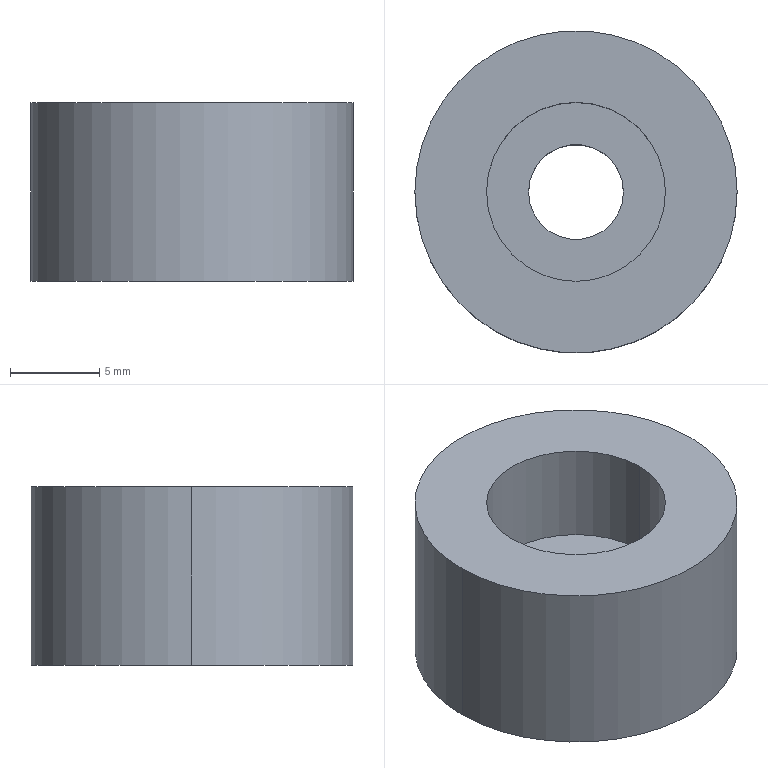Part | STEP file | Buffer block | 1 solid | 9 faces | box 18 x 18 x 10 mm | volume 2002 mm3 | cylinder 6 | plane 3 | commonest cylinder face diameters 5.3 x2 10 x2 18 x2
STEP:
#1=CARTESIAN_POINT('',(0.,0.,0.));
#2=DIRECTION('',(0.,0.,1.));
#3=DIRECTION('',(1.,0.,0.));
#4=AXIS2_PLACEMENT_3D('',#1,#2,#3);
#5=CARTESIAN_POINT('',(5.,0.,4.3));
#6=VERTEX_POINT('',#5);
#7=CARTESIAN_POINT('',(5.,0.,10.));
#8=VERTEX_POINT('',#7);
#9=CARTESIAN_POINT('',(5.,0.,10.));
#10=DIRECTION('',(0.,0.,1.));
#11=VECTOR('',#10,1.);
#12=LINE('',#9,#11);
#13=CARTESIAN_POINT('',(0.,0.,10.));
#14=DIRECTION('',(0.,0.,1.));
#15=DIRECTION('',(1.,0.,0.));
#16=AXIS2_PLACEMENT_3D('',#13,#14,#15);
#17=CYLINDRICAL_SURFACE('',#16,5.);
#18=CARTESIAN_POINT('',(6.283,0.));
#19=DIRECTION('',(0.,1.));
#20=VECTOR('',#19,1.);
#21=LINE('',#18,#20);
#22=(GEOMETRIC_REPRESENTATION_CONTEXT(2)PARAMETRIC_REPRESENTATION_CONTEXT()REPRESENTATION_CONTEXT('',''));
#23=DEFINITIONAL_REPRESENTATION('',(#21),#22);
#24=PCURVE('',#17,#23);
#25=CARTESIAN_POINT('',(0.,0.,10.));
#26=DIRECTION('',(0.,0.,1.));
#27=DIRECTION('',(1.,0.,0.));
#28=AXIS2_PLACEMENT_3D('',#25,#26,#27);
#29=CYLINDRICAL_SURFACE('',#28,5.);
#30=CARTESIAN_POINT('',(0.,0.));
#31=DIRECTION('',(0.,1.));
#32=VECTOR('',#31,1.);
#33=LINE('',#30,#32);
#34=(GEOMETRIC_REPRESENTATION_CONTEXT(2)PARAMETRIC_REPRESENTATION_CONTEXT()REPRESENTATION_CONTEXT('',''));
#35=DEFINITIONAL_REPRESENTATION('',(#33),#34);
#36=PCURVE('',#29,#35);
#37=SURFACE_CURVE('',#12,(#24,#36),.PCURVE_S1.);
#38=EDGE_CURVE('',#6,#8,#37,.T.);
#39=ORIENTED_EDGE('',*,*,#38,.T.);
#40=CARTESIAN_POINT('',(-5.,0.,10.));
#41=VERTEX_POINT('',#40);
#42=CARTESIAN_POINT('',(0.,0.,10.));
#43=DIRECTION('',(0.,0.,1.));
#44=DIRECTION('',(1.,0.,0.));
#45=AXIS2_PLACEMENT_3D('',#42,#43,#44);
#46=CIRCLE('',#45,5.);
#47=CARTESIAN_POINT('',(0.,0.));
#48=DIRECTION('',(1.,0.));
#49=VECTOR('',#48,1.);
#50=LINE('',#47,#49);
#51=(GEOMETRIC_REPRESENTATION_CONTEXT(2)PARAMETRIC_REPRESENTATION_CONTEXT()REPRESENTATION_CONTEXT('',''));
#52=DEFINITIONAL_REPRESENTATION('',(#50),#51);
#53=PCURVE('',#17,#52);
#54=CARTESIAN_POINT('',(0.,0.,10.));
#55=DIRECTION('',(0.,0.,1.));
#56=DIRECTION('',(1.,0.,0.));
#57=AXIS2_PLACEMENT_3D('',#54,#55,#56);
#58=PLANE('',#57);
#59=CARTESIAN_POINT('',(0.,0.));
#60=DIRECTION('',(1.,0.));
#61=AXIS2_PLACEMENT_2D('',#59,#60);
#62=CIRCLE('',#61,5.);
#63=(GEOMETRIC_REPRESENTATION_CONTEXT(2)PARAMETRIC_REPRESENTATION_CONTEXT()REPRESENTATION_CONTEXT('',''));
#64=DEFINITIONAL_REPRESENTATION('',(#62),#63);
#65=PCURVE('',#58,#64);
#66=SURFACE_CURVE('',#46,(#53,#65),.PCURVE_S1.);
#67=EDGE_CURVE('',#41,#8,#66,.T.);
#68=ORIENTED_EDGE('',*,*,#67,.F.);
#69=CARTESIAN_POINT('',(-5.,0.,4.3));
#70=VERTEX_POINT('',#69);
#71=CARTESIAN_POINT('',(-5.,0.,10.));
#72=DIRECTION('',(0.,0.,1.));
#73=VECTOR('',#72,1.);
#74=LINE('',#71,#73);
#75=CARTESIAN_POINT('',(3.142,0.));
#76=DIRECTION('',(0.,1.));
#77=VECTOR('',#76,1.);
#78=LINE('',#75,#77);
#79=(GEOMETRIC_REPRESENTATION_CONTEXT(2)PARAMETRIC_REPRESENTATION_CONTEXT()REPRESENTATION_CONTEXT('',''));
#80=DEFINITIONAL_REPRESENTATION('',(#78),#79);
#81=PCURVE('',#17,#80);
#82=CARTESIAN_POINT('',(3.142,0.));
#83=DIRECTION('',(0.,1.));
#84=VECTOR('',#83,1.);
#85=LINE('',#82,#84);
#86=(GEOMETRIC_REPRESENTATION_CONTEXT(2)PARAMETRIC_REPRESENTATION_CONTEXT()REPRESENTATION_CONTEXT('',''));
#87=DEFINITIONAL_REPRESENTATION('',(#85),#86);
#88=PCURVE('',#29,#87);
#89=SURFACE_CURVE('',#74,(#81,#88),.PCURVE_S1.);
#90=EDGE_CURVE('',#70,#41,#89,.T.);
#91=ORIENTED_EDGE('',*,*,#90,.F.);
#92=CARTESIAN_POINT('',(0.,0.,4.3));
#93=DIRECTION('',(0.,0.,1.));
#94=DIRECTION('',(1.,0.,0.));
#95=AXIS2_PLACEMENT_3D('',#92,#93,#94);
#96=CIRCLE('',#95,5.);
#97=CARTESIAN_POINT('',(0.,-5.7));
#98=DIRECTION('',(1.,0.));
#99=VECTOR('',#98,1.);
#100=LINE('',#97,#99);
#101=(GEOMETRIC_REPRESENTATION_CONTEXT(2)PARAMETRIC_REPRESENTATION_CONTEXT()REPRESENTATION_CONTEXT('',''));
#102=DEFINITIONAL_REPRESENTATION('',(#100),#101);
#103=PCURVE('',#17,#102);
#104=CARTESIAN_POINT('',(2.65,0.,4.3));
#105=DIRECTION('',(0.,0.,-1.));
#106=DIRECTION('',(-1.,0.,0.));
#107=AXIS2_PLACEMENT_3D('',#104,#105,#106);
#108=PLANE('',#107);
#109=CARTESIAN_POINT('',(-2.35,0.));
#110=CARTESIAN_POINT('',(-2.35,8.66));
#111=CARTESIAN_POINT('',(5.15,4.33));
#112=CARTESIAN_POINT('',(12.65,0.));
#113=CARTESIAN_POINT('',(5.15,-4.33));
#114=CARTESIAN_POINT('',(-2.35,-8.66));
#115=CARTESIAN_POINT('',(-2.35,0.));
#116=(BOUNDED_CURVE()B_SPLINE_CURVE(2,(#109,#110,#111,#112,#113,#114,#115),.UNSPECIFIED.,.T.,.F.)B_SPLINE_CURVE_WITH_KNOTS((1,2,2,2,2,1),(-2.094,0.,2.094,4.189,6.283,8.378),.UNSPECIFIED.)CURVE()GEOMETRIC_REPRESENTATION_ITEM()RATIONAL_B_SPLINE_CURVE((1.,0.5,1.,0.5,1.,0.5,1.))REPRESENTATION_ITEM(''));
#117=(GEOMETRIC_REPRESENTATION_CONTEXT(2)PARAMETRIC_REPRESENTATION_CONTEXT()REPRESENTATION_CONTEXT('',''));
#118=DEFINITIONAL_REPRESENTATION('',(#116),#117);
#119=PCURVE('',#108,#118);
#120=SURFACE_CURVE('',#96,(#103,#119),.PCURVE_S1.);
#121=EDGE_CURVE('',#70,#6,#120,.T.);
#122=ORIENTED_EDGE('',*,*,#121,.T.);
#123=EDGE_LOOP('',(#39,#68,#91,#122));
#124=FACE_BOUND('',#123,.F.);
#125=ADVANCED_FACE('',(#124),#17,.F.);
#126=CARTESIAN_POINT('',(2.65,0.,0.));
#127=VERTEX_POINT('',#126);
#128=CARTESIAN_POINT('',(2.65,0.,4.3));
#129=VERTEX_POINT('',#128);
#130=CARTESIAN_POINT('',(2.65,0.,10.));
#131=DIRECTION('',(0.,0.,1.));
#132=VECTOR('',#131,1.);
#133=LINE('',#130,#132);
#134=CARTESIAN_POINT('',(0.,0.,10.));
#135=DIRECTION('',(0.,0.,1.));
#136=DIRECTION('',(1.,0.,0.));
#137=AXIS2_PLACEMENT_3D('',#134,#135,#136);
#138=CYLINDRICAL_SURFACE('',#137,2.65);
#139=CARTESIAN_POINT('',(6.283,0.));
#140=DIRECTION('',(0.,1.));
#141=VECTOR('',#140,1.);
#142=LINE('',#139,#141);
#143=(GEOMETRIC_REPRESENTATION_CONTEXT(2)PARAMETRIC_REPRESENTATION_CONTEXT()REPRESENTATION_CONTEXT('',''));
#144=DEFINITIONAL_REPRESENTATION('',(#142),#143);
#145=PCURVE('',#138,#144);
#146=CARTESIAN_POINT('',(0.,0.,10.));
#147=DIRECTION('',(0.,0.,1.));
#148=DIRECTION('',(1.,0.,0.));
#149=AXIS2_PLACEMENT_3D('',#146,#147,#148);
#150=CYLINDRICAL_SURFACE('',#149,2.65);
#151=CARTESIAN_POINT('',(0.,0.));
#152=DIRECTION('',(0.,1.));
#153=VECTOR('',#152,1.);
#154=LINE('',#151,#153);
#155=(GEOMETRIC_REPRESENTATION_CONTEXT(2)PARAMETRIC_REPRESENTATION_CONTEXT()REPRESENTATION_CONTEXT('',''));
#156=DEFINITIONAL_REPRESENTATION('',(#154),#155);
#157=PCURVE('',#150,#156);
#158=SURFACE_CURVE('',#133,(#145,#157),.PCURVE_S1.);
#159=EDGE_CURVE('',#127,#129,#158,.T.);
#160=ORIENTED_EDGE('',*,*,#159,.T.);
#161=CARTESIAN_POINT('',(-2.65,0.,4.3));
#162=VERTEX_POINT('',#161);
#163=CARTESIAN_POINT('',(0.,0.,4.3));
#164=DIRECTION('',(0.,0.,1.));
#165=DIRECTION('',(1.,0.,0.));
#166=AXIS2_PLACEMENT_3D('',#163,#164,#165);
#167=CIRCLE('',#166,2.65);
#168=CARTESIAN_POINT('',(0.,-5.7));
#169=DIRECTION('',(1.,0.));
#170=VECTOR('',#169,1.);
#171=LINE('',#168,#170);
#172=(GEOMETRIC_REPRESENTATION_CONTEXT(2)PARAMETRIC_REPRESENTATION_CONTEXT()REPRESENTATION_CONTEXT('',''));
#173=DEFINITIONAL_REPRESENTATION('',(#171),#172);
#174=PCURVE('',#138,#173);
#175=CARTESIAN_POINT('',(0.,0.));
#176=CARTESIAN_POINT('',(0.,4.59));
#177=CARTESIAN_POINT('',(3.975,2.295));
#178=CARTESIAN_POINT('',(7.95,0.));
#179=CARTESIAN_POINT('',(3.975,-2.295));
#180=CARTESIAN_POINT('',(0.,-4.59));
#181=CARTESIAN_POINT('',(0.,0.));
#182=(BOUNDED_CURVE()B_SPLINE_CURVE(2,(#175,#176,#177,#178,#179,#180,#181),.UNSPECIFIED.,.T.,.F.)B_SPLINE_CURVE_WITH_KNOTS((1,2,2,2,2,1),(-2.094,0.,2.094,4.189,6.283,8.378),.UNSPECIFIED.)CURVE()GEOMETRIC_REPRESENTATION_ITEM()RATIONAL_B_SPLINE_CURVE((1.,0.5,1.,0.5,1.,0.5,1.))REPRESENTATION_ITEM(''));
#183=(GEOMETRIC_REPRESENTATION_CONTEXT(2)PARAMETRIC_REPRESENTATION_CONTEXT()REPRESENTATION_CONTEXT('',''));
#184=DEFINITIONAL_REPRESENTATION('',(#182),#183);
#185=PCURVE('',#108,#184);
#186=SURFACE_CURVE('',#167,(#174,#185),.PCURVE_S1.);
#187=EDGE_CURVE('',#162,#129,#186,.T.);
#188=ORIENTED_EDGE('',*,*,#187,.F.);
#189=CARTESIAN_POINT('',(-2.65,0.,0.));
#190=VERTEX_POINT('',#189);
#191=CARTESIAN_POINT('',(-2.65,0.,10.));
#192=DIRECTION('',(0.,0.,1.));
#193=VECTOR('',#192,1.);
#194=LINE('',#191,#193);
#195=CARTESIAN_POINT('',(3.142,0.));
#196=DIRECTION('',(0.,1.));
#197=VECTOR('',#196,1.);
#198=LINE('',#195,#197);
#199=(GEOMETRIC_REPRESENTATION_CONTEXT(2)PARAMETRIC_REPRESENTATION_CONTEXT()REPRESENTATION_CONTEXT('',''));
#200=DEFINITIONAL_REPRESENTATION('',(#198),#199);
#201=PCURVE('',#138,#200);
#202=CARTESIAN_POINT('',(3.142,0.));
#203=DIRECTION('',(0.,1.));
#204=VECTOR('',#203,1.);
#205=LINE('',#202,#204);
#206=(GEOMETRIC_REPRESENTATION_CONTEXT(2)PARAMETRIC_REPRESENTATION_CONTEXT()REPRESENTATION_CONTEXT('',''));
#207=DEFINITIONAL_REPRESENTATION('',(#205),#206);
#208=PCURVE('',#150,#207);
#209=SURFACE_CURVE('',#194,(#201,#208),.PCURVE_S1.);
#210=EDGE_CURVE('',#190,#162,#209,.T.);
#211=ORIENTED_EDGE('',*,*,#210,.F.);
#212=CARTESIAN_POINT('',(0.,0.,0.));
#213=DIRECTION('',(0.,0.,1.));
#214=DIRECTION('',(1.,0.,0.));
#215=AXIS2_PLACEMENT_3D('',#212,#213,#214);
#216=CIRCLE('',#215,2.65);
#217=CARTESIAN_POINT('',(0.,-10.));
#218=DIRECTION('',(1.,0.));
#219=VECTOR('',#218,1.);
#220=LINE('',#217,#219);
#221=(GEOMETRIC_REPRESENTATION_CONTEXT(2)PARAMETRIC_REPRESENTATION_CONTEXT()REPRESENTATION_CONTEXT('',''));
#222=DEFINITIONAL_REPRESENTATION('',(#220),#221);
#223=PCURVE('',#138,#222);
#224=CARTESIAN_POINT('',(0.,0.,0.));
#225=DIRECTION('',(0.,0.,1.));
#226=DIRECTION('',(1.,0.,0.));
#227=AXIS2_PLACEMENT_3D('',#224,#225,#226);
#228=PLANE('',#227);
#229=CARTESIAN_POINT('',(0.,0.));
#230=DIRECTION('',(1.,0.));
#231=AXIS2_PLACEMENT_2D('',#229,#230);
#232=CIRCLE('',#231,2.65);
#233=(GEOMETRIC_REPRESENTATION_CONTEXT(2)PARAMETRIC_REPRESENTATION_CONTEXT()REPRESENTATION_CONTEXT('',''));
#234=DEFINITIONAL_REPRESENTATION('',(#232),#233);
#235=PCURVE('',#228,#234);
#236=SURFACE_CURVE('',#216,(#223,#235),.PCURVE_S1.);
#237=EDGE_CURVE('',#190,#127,#236,.T.);
#238=ORIENTED_EDGE('',*,*,#237,.T.);
#239=EDGE_LOOP('',(#160,#188,#211,#238));
#240=FACE_BOUND('',#239,.F.);
#241=ADVANCED_FACE('',(#240),#138,.F.);
#242=CARTESIAN_POINT('',(9.,0.,10.));
#243=VERTEX_POINT('',#242);
#244=CARTESIAN_POINT('',(-9.,0.,10.));
#245=VERTEX_POINT('',#244);
#246=CARTESIAN_POINT('',(0.,0.,10.));
#247=DIRECTION('',(0.,0.,1.));
#248=DIRECTION('',(1.,0.,0.));
#249=AXIS2_PLACEMENT_3D('',#246,#247,#248);
#250=CIRCLE('',#249,9.);
#251=CARTESIAN_POINT('',(0.,0.,10.));
#252=DIRECTION('',(0.,0.,-1.));
#253=DIRECTION('',(-1.,0.,0.));
#254=AXIS2_PLACEMENT_3D('',#251,#252,#253);
#255=CYLINDRICAL_SURFACE('',#254,9.);
#256=CARTESIAN_POINT('',(3.142,0.));
#257=DIRECTION('',(-1.,0.));
#258=VECTOR('',#257,1.);
#259=LINE('',#256,#258);
#260=(GEOMETRIC_REPRESENTATION_CONTEXT(2)PARAMETRIC_REPRESENTATION_CONTEXT()REPRESENTATION_CONTEXT('',''));
#261=DEFINITIONAL_REPRESENTATION('',(#259),#260);
#262=PCURVE('',#255,#261);
#263=CARTESIAN_POINT('',(0.,0.));
#264=DIRECTION('',(1.,0.));
#265=AXIS2_PLACEMENT_2D('',#263,#264);
#266=CIRCLE('',#265,9.);
#267=(GEOMETRIC_REPRESENTATION_CONTEXT(2)PARAMETRIC_REPRESENTATION_CONTEXT()REPRESENTATION_CONTEXT('',''));
#268=DEFINITIONAL_REPRESENTATION('',(#266),#267);
#269=PCURVE('',#58,#268);
#270=SURFACE_CURVE('',#250,(#262,#269),.PCURVE_S1.);
#271=EDGE_CURVE('',#243,#245,#270,.T.);
#272=ORIENTED_EDGE('',*,*,#271,.F.);
#273=CARTESIAN_POINT('',(9.,0.,0.));
#274=VERTEX_POINT('',#273);
#275=CARTESIAN_POINT('',(9.,0.,10.));
#276=DIRECTION('',(0.,0.,-1.));
#277=VECTOR('',#276,1.);
#278=LINE('',#275,#277);
#279=CARTESIAN_POINT('',(3.142,0.));
#280=DIRECTION('',(0.,1.));
#281=VECTOR('',#280,1.);
#282=LINE('',#279,#281);
#283=(GEOMETRIC_REPRESENTATION_CONTEXT(2)PARAMETRIC_REPRESENTATION_CONTEXT()REPRESENTATION_CONTEXT('',''));
#284=DEFINITIONAL_REPRESENTATION('',(#282),#283);
#285=PCURVE('',#255,#284);
#286=CARTESIAN_POINT('',(0.,0.,10.));
#287=DIRECTION('',(0.,0.,-1.));
#288=DIRECTION('',(-1.,0.,0.));
#289=AXIS2_PLACEMENT_3D('',#286,#287,#288);
#290=CYLINDRICAL_SURFACE('',#289,9.);
#291=CARTESIAN_POINT('',(3.142,0.));
#292=DIRECTION('',(0.,1.));
#293=VECTOR('',#292,1.);
#294=LINE('',#291,#293);
#295=(GEOMETRIC_REPRESENTATION_CONTEXT(2)PARAMETRIC_REPRESENTATION_CONTEXT()REPRESENTATION_CONTEXT('',''));
#296=DEFINITIONAL_REPRESENTATION('',(#294),#295);
#297=PCURVE('',#290,#296);
#298=SURFACE_CURVE('',#278,(#285,#297),.PCURVE_S1.);
#299=EDGE_CURVE('',#243,#274,#298,.T.);
#300=ORIENTED_EDGE('',*,*,#299,.T.);
#301=CARTESIAN_POINT('',(-9.,0.,0.));
#302=VERTEX_POINT('',#301);
#303=CARTESIAN_POINT('',(0.,0.,0.));
#304=DIRECTION('',(0.,0.,1.));
#305=DIRECTION('',(1.,0.,0.));
#306=AXIS2_PLACEMENT_3D('',#303,#304,#305);
#307=CIRCLE('',#306,9.);
#308=CARTESIAN_POINT('',(3.142,10.));
#309=DIRECTION('',(-1.,0.));
#310=VECTOR('',#309,1.);
#311=LINE('',#308,#310);
#312=(GEOMETRIC_REPRESENTATION_CONTEXT(2)PARAMETRIC_REPRESENTATION_CONTEXT()REPRESENTATION_CONTEXT('',''));
#313=DEFINITIONAL_REPRESENTATION('',(#311),#312);
#314=PCURVE('',#255,#313);
#315=CARTESIAN_POINT('',(0.,0.));
#316=DIRECTION('',(1.,0.));
#317=AXIS2_PLACEMENT_2D('',#315,#316);
#318=CIRCLE('',#317,9.);
#319=(GEOMETRIC_REPRESENTATION_CONTEXT(2)PARAMETRIC_REPRESENTATION_CONTEXT()REPRESENTATION_CONTEXT('',''));
#320=DEFINITIONAL_REPRESENTATION('',(#318),#319);
#321=PCURVE('',#228,#320);
#322=SURFACE_CURVE('',#307,(#314,#321),.PCURVE_S1.);
#323=EDGE_CURVE('',#274,#302,#322,.T.);
#324=ORIENTED_EDGE('',*,*,#323,.T.);
#325=CARTESIAN_POINT('',(-9.,0.,10.));
#326=DIRECTION('',(0.,0.,-1.));
#327=VECTOR('',#326,1.);
#328=LINE('',#325,#327);
#329=CARTESIAN_POINT('',(0.,0.));
#330=DIRECTION('',(0.,1.));
#331=VECTOR('',#330,1.);
#332=LINE('',#329,#331);
#333=(GEOMETRIC_REPRESENTATION_CONTEXT(2)PARAMETRIC_REPRESENTATION_CONTEXT()REPRESENTATION_CONTEXT('',''));
#334=DEFINITIONAL_REPRESENTATION('',(#332),#333);
#335=PCURVE('',#255,#334);
#336=CARTESIAN_POINT('',(6.283,0.));
#337=DIRECTION('',(0.,1.));
#338=VECTOR('',#337,1.);
#339=LINE('',#336,#338);
#340=(GEOMETRIC_REPRESENTATION_CONTEXT(2)PARAMETRIC_REPRESENTATION_CONTEXT()REPRESENTATION_CONTEXT('',''));
#341=DEFINITIONAL_REPRESENTATION('',(#339),#340);
#342=PCURVE('',#290,#341);
#343=SURFACE_CURVE('',#328,(#335,#342),.PCURVE_S1.);
#344=EDGE_CURVE('',#245,#302,#343,.T.);
#345=ORIENTED_EDGE('',*,*,#344,.F.);
#346=EDGE_LOOP('',(#272,#300,#324,#345));
#347=FACE_BOUND('',#346,.T.);
#348=ADVANCED_FACE('',(#347),#255,.T.);
#349=ORIENTED_EDGE('',*,*,#299,.F.);
#350=CARTESIAN_POINT('',(0.,0.,10.));
#351=DIRECTION('',(0.,0.,1.));
#352=DIRECTION('',(1.,0.,0.));
#353=AXIS2_PLACEMENT_3D('',#350,#351,#352);
#354=CIRCLE('',#353,9.);
#355=CARTESIAN_POINT('',(9.425,0.));
#356=DIRECTION('',(-1.,0.));
#357=VECTOR('',#356,1.);
#358=LINE('',#355,#357);
#359=(GEOMETRIC_REPRESENTATION_CONTEXT(2)PARAMETRIC_REPRESENTATION_CONTEXT()REPRESENTATION_CONTEXT('',''));
#360=DEFINITIONAL_REPRESENTATION('',(#358),#359);
#361=PCURVE('',#290,#360);
#362=CARTESIAN_POINT('',(0.,0.));
#363=DIRECTION('',(1.,0.));
#364=AXIS2_PLACEMENT_2D('',#362,#363);
#365=CIRCLE('',#364,9.);
#366=(GEOMETRIC_REPRESENTATION_CONTEXT(2)PARAMETRIC_REPRESENTATION_CONTEXT()REPRESENTATION_CONTEXT('',''));
#367=DEFINITIONAL_REPRESENTATION('',(#365),#366);
#368=PCURVE('',#58,#367);
#369=SURFACE_CURVE('',#354,(#361,#368),.PCURVE_S1.);
#370=EDGE_CURVE('',#245,#243,#369,.T.);
#371=ORIENTED_EDGE('',*,*,#370,.F.);
#372=ORIENTED_EDGE('',*,*,#344,.T.);
#373=CARTESIAN_POINT('',(0.,0.,0.));
#374=DIRECTION('',(0.,0.,1.));
#375=DIRECTION('',(1.,0.,0.));
#376=AXIS2_PLACEMENT_3D('',#373,#374,#375);
#377=CIRCLE('',#376,9.);
#378=CARTESIAN_POINT('',(9.425,10.));
#379=DIRECTION('',(-1.,0.));
#380=VECTOR('',#379,1.);
#381=LINE('',#378,#380);
#382=(GEOMETRIC_REPRESENTATION_CONTEXT(2)PARAMETRIC_REPRESENTATION_CONTEXT()REPRESENTATION_CONTEXT('',''));
#383=DEFINITIONAL_REPRESENTATION('',(#381),#382);
#384=PCURVE('',#290,#383);
#385=CARTESIAN_POINT('',(0.,0.));
#386=DIRECTION('',(1.,0.));
#387=AXIS2_PLACEMENT_2D('',#385,#386);
#388=CIRCLE('',#387,9.);
#389=(GEOMETRIC_REPRESENTATION_CONTEXT(2)PARAMETRIC_REPRESENTATION_CONTEXT()REPRESENTATION_CONTEXT('',''));
#390=DEFINITIONAL_REPRESENTATION('',(#388),#389);
#391=PCURVE('',#228,#390);
#392=SURFACE_CURVE('',#377,(#384,#391),.PCURVE_S1.);
#393=EDGE_CURVE('',#302,#274,#392,.T.);
#394=ORIENTED_EDGE('',*,*,#393,.T.);
#395=EDGE_LOOP('',(#349,#371,#372,#394));
#396=FACE_BOUND('',#395,.T.);
#397=ADVANCED_FACE('',(#396),#290,.T.);
#398=CARTESIAN_POINT('',(0.,0.,10.));
#399=DIRECTION('',(0.,0.,1.));
#400=DIRECTION('',(1.,0.,0.));
#401=AXIS2_PLACEMENT_3D('',#398,#399,#400);
#402=CIRCLE('',#401,5.);
#403=CARTESIAN_POINT('',(0.,0.));
#404=DIRECTION('',(1.,0.));
#405=AXIS2_PLACEMENT_2D('',#403,#404);
#406=CIRCLE('',#405,5.);
#407=(GEOMETRIC_REPRESENTATION_CONTEXT(2)PARAMETRIC_REPRESENTATION_CONTEXT()REPRESENTATION_CONTEXT('',''));
#408=DEFINITIONAL_REPRESENTATION('',(#406),#407);
#409=PCURVE('',#58,#408);
#410=CARTESIAN_POINT('',(0.,0.));
#411=DIRECTION('',(1.,0.));
#412=VECTOR('',#411,1.);
#413=LINE('',#410,#412);
#414=(GEOMETRIC_REPRESENTATION_CONTEXT(2)PARAMETRIC_REPRESENTATION_CONTEXT()REPRESENTATION_CONTEXT('',''));
#415=DEFINITIONAL_REPRESENTATION('',(#413),#414);
#416=PCURVE('',#29,#415);
#417=SURFACE_CURVE('',#402,(#409,#416),.PCURVE_S1.);
#418=EDGE_CURVE('',#8,#41,#417,.T.);
#419=ORIENTED_EDGE('',*,*,#418,.F.);
#420=ORIENTED_EDGE('',*,*,#67,.F.);
#421=EDGE_LOOP('',(#419,#420));
#422=FACE_BOUND('',#421,.T.);
#423=ORIENTED_EDGE('',*,*,#370,.T.);
#424=ORIENTED_EDGE('',*,*,#271,.T.);
#425=EDGE_LOOP('',(#423,#424));
#426=FACE_BOUND('',#425,.T.);
#427=ADVANCED_FACE('',(#422,#426),#58,.T.);
#428=CARTESIAN_POINT('',(0.,0.,0.));
#429=DIRECTION('',(0.,0.,1.));
#430=DIRECTION('',(1.,0.,0.));
#431=AXIS2_PLACEMENT_3D('',#428,#429,#430);
#432=CIRCLE('',#431,2.65);
#433=CARTESIAN_POINT('',(0.,0.));
#434=DIRECTION('',(1.,0.));
#435=AXIS2_PLACEMENT_2D('',#433,#434);
#436=CIRCLE('',#435,2.65);
#437=(GEOMETRIC_REPRESENTATION_CONTEXT(2)PARAMETRIC_REPRESENTATION_CONTEXT()REPRESENTATION_CONTEXT('',''));
#438=DEFINITIONAL_REPRESENTATION('',(#436),#437);
#439=PCURVE('',#228,#438);
#440=CARTESIAN_POINT('',(0.,-10.));
#441=DIRECTION('',(1.,0.));
#442=VECTOR('',#441,1.);
#443=LINE('',#440,#442);
#444=(GEOMETRIC_REPRESENTATION_CONTEXT(2)PARAMETRIC_REPRESENTATION_CONTEXT()REPRESENTATION_CONTEXT('',''));
#445=DEFINITIONAL_REPRESENTATION('',(#443),#444);
#446=PCURVE('',#150,#445);
#447=SURFACE_CURVE('',#432,(#439,#446),.PCURVE_S1.);
#448=EDGE_CURVE('',#127,#190,#447,.T.);
#449=ORIENTED_EDGE('',*,*,#448,.T.);
#450=ORIENTED_EDGE('',*,*,#237,.T.);
#451=EDGE_LOOP('',(#449,#450));
#452=FACE_BOUND('',#451,.T.);
#453=ORIENTED_EDGE('',*,*,#393,.F.);
#454=ORIENTED_EDGE('',*,*,#323,.F.);
#455=EDGE_LOOP('',(#453,#454));
#456=FACE_BOUND('',#455,.T.);
#457=ADVANCED_FACE('',(#452,#456),#228,.F.);
#458=CARTESIAN_POINT('',(0.,0.,4.3));
#459=DIRECTION('',(0.,0.,1.));
#460=DIRECTION('',(1.,0.,0.));
#461=AXIS2_PLACEMENT_3D('',#458,#459,#460);
#462=CIRCLE('',#461,2.65);
#463=CARTESIAN_POINT('',(0.,-5.7));
#464=DIRECTION('',(1.,0.));
#465=VECTOR('',#464,1.);
#466=LINE('',#463,#465);
#467=(GEOMETRIC_REPRESENTATION_CONTEXT(2)PARAMETRIC_REPRESENTATION_CONTEXT()REPRESENTATION_CONTEXT('',''));
#468=DEFINITIONAL_REPRESENTATION('',(#466),#467);
#469=PCURVE('',#150,#468);
#470=CARTESIAN_POINT('',(0.,0.));
#471=CARTESIAN_POINT('',(0.,4.59));
#472=CARTESIAN_POINT('',(3.975,2.295));
#473=CARTESIAN_POINT('',(7.95,0.));
#474=CARTESIAN_POINT('',(3.975,-2.295));
#475=CARTESIAN_POINT('',(0.,-4.59));
#476=CARTESIAN_POINT('',(0.,0.));
#477=(BOUNDED_CURVE()B_SPLINE_CURVE(2,(#470,#471,#472,#473,#474,#475,#476),.UNSPECIFIED.,.T.,.F.)B_SPLINE_CURVE_WITH_KNOTS((1,2,2,2,2,1),(-2.094,0.,2.094,4.189,6.283,8.378),.UNSPECIFIED.)CURVE()GEOMETRIC_REPRESENTATION_ITEM()RATIONAL_B_SPLINE_CURVE((1.,0.5,1.,0.5,1.,0.5,1.))REPRESENTATION_ITEM(''));
#478=(GEOMETRIC_REPRESENTATION_CONTEXT(2)PARAMETRIC_REPRESENTATION_CONTEXT()REPRESENTATION_CONTEXT('',''));
#479=DEFINITIONAL_REPRESENTATION('',(#477),#478);
#480=PCURVE('',#108,#479);
#481=SURFACE_CURVE('',#462,(#469,#480),.PCURVE_S1.);
#482=EDGE_CURVE('',#129,#162,#481,.T.);
#483=ORIENTED_EDGE('',*,*,#482,.F.);
#484=ORIENTED_EDGE('',*,*,#159,.F.);
#485=ORIENTED_EDGE('',*,*,#448,.T.);
#486=ORIENTED_EDGE('',*,*,#210,.T.);
#487=EDGE_LOOP('',(#483,#484,#485,#486));
#488=FACE_BOUND('',#487,.F.);
#489=ADVANCED_FACE('',(#488),#150,.F.);
#490=ORIENTED_EDGE('',*,*,#482,.F.);
#491=ORIENTED_EDGE('',*,*,#187,.F.);
#492=EDGE_LOOP('',(#490,#491));
#493=FACE_BOUND('',#492,.T.);
#494=CARTESIAN_POINT('',(0.,0.,4.3));
#495=DIRECTION('',(0.,0.,1.));
#496=DIRECTION('',(1.,0.,0.));
#497=AXIS2_PLACEMENT_3D('',#494,#495,#496);
#498=CIRCLE('',#497,5.);
#499=CARTESIAN_POINT('',(-2.35,0.));
#500=CARTESIAN_POINT('',(-2.35,8.66));
#501=CARTESIAN_POINT('',(5.15,4.33));
#502=CARTESIAN_POINT('',(12.65,0.));
#503=CARTESIAN_POINT('',(5.15,-4.33));
#504=CARTESIAN_POINT('',(-2.35,-8.66));
#505=CARTESIAN_POINT('',(-2.35,0.));
#506=(BOUNDED_CURVE()B_SPLINE_CURVE(2,(#499,#500,#501,#502,#503,#504,#505),.UNSPECIFIED.,.T.,.F.)B_SPLINE_CURVE_WITH_KNOTS((1,2,2,2,2,1),(-2.094,0.,2.094,4.189,6.283,8.378),.UNSPECIFIED.)CURVE()GEOMETRIC_REPRESENTATION_ITEM()RATIONAL_B_SPLINE_CURVE((1.,0.5,1.,0.5,1.,0.5,1.))REPRESENTATION_ITEM(''));
#507=(GEOMETRIC_REPRESENTATION_CONTEXT(2)PARAMETRIC_REPRESENTATION_CONTEXT()REPRESENTATION_CONTEXT('',''));
#508=DEFINITIONAL_REPRESENTATION('',(#506),#507);
#509=PCURVE('',#108,#508);
#510=CARTESIAN_POINT('',(0.,-5.7));
#511=DIRECTION('',(1.,0.));
#512=VECTOR('',#511,1.);
#513=LINE('',#510,#512);
#514=(GEOMETRIC_REPRESENTATION_CONTEXT(2)PARAMETRIC_REPRESENTATION_CONTEXT()REPRESENTATION_CONTEXT('',''));
#515=DEFINITIONAL_REPRESENTATION('',(#513),#514);
#516=PCURVE('',#29,#515);
#517=SURFACE_CURVE('',#498,(#509,#516),.PCURVE_S1.);
#518=EDGE_CURVE('',#6,#70,#517,.T.);
#519=ORIENTED_EDGE('',*,*,#518,.T.);
#520=ORIENTED_EDGE('',*,*,#121,.T.);
#521=EDGE_LOOP('',(#519,#520));
#522=FACE_BOUND('',#521,.T.);
#523=ADVANCED_FACE('',(#493,#522),#108,.F.);
#524=ORIENTED_EDGE('',*,*,#418,.F.);
#525=ORIENTED_EDGE('',*,*,#38,.F.);
#526=ORIENTED_EDGE('',*,*,#518,.T.);
#527=ORIENTED_EDGE('',*,*,#90,.T.);
#528=EDGE_LOOP('',(#524,#525,#526,#527));
#529=FACE_BOUND('',#528,.F.);
#530=ADVANCED_FACE('',(#529),#29,.F.);
#531=CLOSED_SHELL('',(#125,#241,#348,#397,#427,#457,#489,#523,#530));
#532=MANIFOLD_SOLID_BREP('',#531);
#533=(LENGTH_UNIT()NAMED_UNIT(*)SI_UNIT(.MILLI.,.METRE.));
#534=UNCERTAINTY_MEASURE_WITH_UNIT(LENGTH_MEASURE(0.0000001),#533,'','');
#535=(NAMED_UNIT(*)PLANE_ANGLE_UNIT()SI_UNIT($,.RADIAN.));
#536=(NAMED_UNIT(*)SI_UNIT($,.STERADIAN.)SOLID_ANGLE_UNIT());
#537=(GEOMETRIC_REPRESENTATION_CONTEXT(3)GLOBAL_UNCERTAINTY_ASSIGNED_CONTEXT((#534))GLOBAL_UNIT_ASSIGNED_CONTEXT((#533,#535,#536))REPRESENTATION_CONTEXT('',''));
#538=ADVANCED_BREP_SHAPE_REPRESENTATION('',(#4,#532),#537);